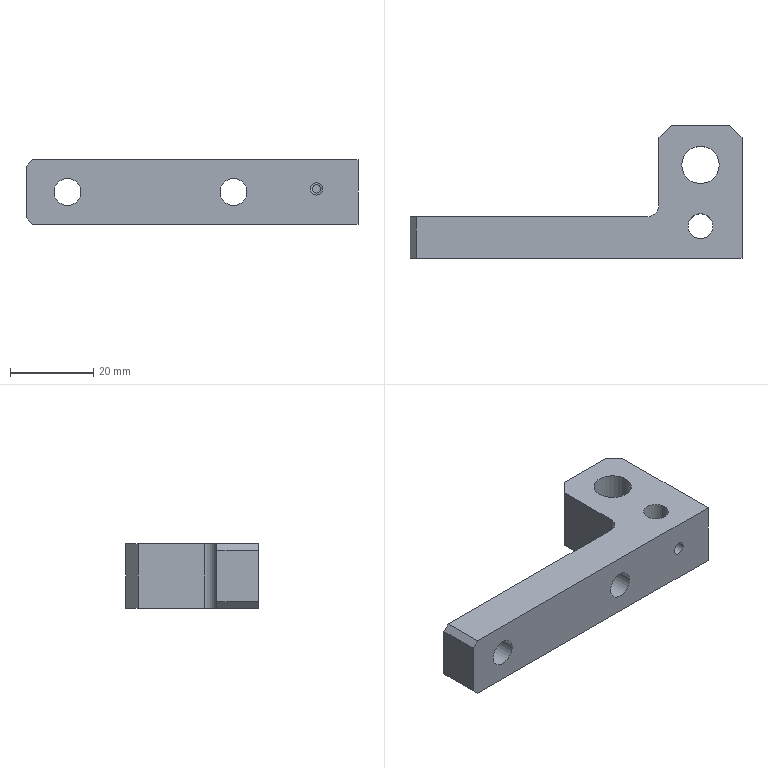NC program | NX | posted with a generic post | part box 80 x 32 x 15.5 mm
Whole program:
N10 G17 G21 G94 G90
(PLANAR_MILL_7 , TOOL : D10-30-D10-75-3T-ROUGH)
N12 T01 M6
N14 G54
N16 G17 G0 G90 X-37.156 Y-16.306 B0. C0. S3000 M3
N18 G43 Z20. H1
N20 Z-9. B-180. C-180.
N22 G94 G1 Z-11. F800.
N24 X-42.106 Y-11.356
N26 X-43.606 Y-9.856
N28 X-48.556 Y-4.906
N30 Z-9.
N32 G0 Z20.
N34 Y4.906
N36 Z-9.
N38 G1 Z-11.
N40 X-43.606 Y9.856
N42 X-42.106 Y11.356
N44 X-37.156 Y16.306
N46 Z-9.
N48 G0 Z20.
N50 M5
(PLANAR_MILL_7_COPY , TOOL : D6-18-D6-50-3T-FINISH)
N52 T06 M6
N54 G54
N56 G17 G0 G90 X-37.086 Y-13.407 B0. C0. S3000 M3
N58 G43 Z20. H6
N60 Z-9. B-180. C-180.
N62 G94 G1 Z-11. F600.
N64 X-40.621 Y-9.871
N66 X-42.121 Y-8.371
N68 X-45.657 Y-4.836
N70 Z-9.
N72 G0 Z20.
N74 Y4.836
N76 Z-9.
N78 G1 Z-11.
N80 X-42.121 Y8.371
N82 X-40.621 Y9.871
N84 X-37.086 Y13.407
N86 Z-9.
N88 G0 Z20.
N90 M5
(DRILLING_3 , TOOL : 点孔D10-150-90度)
N92 T02 M6
N94 G54
N96 G17 G0 G90 X30. Y0.75 B0. C0. S1600 M3
N98 G43 Z20. H2
N100 G94 G81 G99 Z-1. B-180. C-180. F60. R3.
N102 G80
N104 G0 X30. Y0.75 Z20.
(DRILLING_3_COPY_2 , TOOL : 点孔D10-150-90度)
N106 X-30. Y0.
N108 G81 Z-1. F60. R3.
N110 X10.
N112 G80
N114 G0 X10. Y0. Z20.
N116 M5
(DRILLING_3_COPY , TOOL : 钻头D3.0-42-71)
N118 T16 M6
N120 G54
N122 G17 G0 G90 X30. Y0.75 B0. C0. S1600 M3
N124 G43 Z20. H16
N126 G94 G83 G99 Z-11. B-180. C-180. F60. Q1. R3.
N128 G80
N130 G0 X30. Y0.75 Z20.
N132 M5
(DRILLING_3_COPY_COPY , TOOL : 钻头D2.0-29-55)
N134 T14 M6
N136 G54
N138 G17 G0 G90 X30. Y0.75 B0. C0. S1600 M3
N140 G43 Z20. H14
N142 G94 G83 G99 Z-20. B-180. C-180. F30. Q0.5 R3.
N144 G80
N146 G0 X30. Y0.75 Z20.
N148 M5
(DRILLING_3_COPY_1 , TOOL : 钻头D6.5-73-105)
N150 T15 M6
N152 G54
N154 G17 G0 G90 X-30. Y0. B0. C0. S1200 M3
N156 G43 Z20. H15
N158 G94 G83 G99 Z-13. B-180. C-180. F60. Q1.5 R3.
N160 X10.
N162 G80
N164 G0 X10. Y0. Z20.
N166 M5
(DRILLING_3_COPY_3 , TOOL : 点孔D10-150-90度)
N168 T02 M6
N170 G54
N172 G17 G0 G90 X30. Y0.75 B0. C0. S1600 M3
N174 G43 Z20. H2
N176 G94 G81 G99 Z-1.5 B-180. C-180. F60. R3.
N178 G80
N180 G0 X30. Y0.75 Z20.
(DRILLING_3_COPY_2_COPY , TOOL : 点孔D10-150-90度)
N182 X-30. Y0.
N184 G81 Z-3.25 F60. R3.
N186 X10.
N188 G80
N190 G0 X10. Y0. Z20.
N192 M5
N194 M2